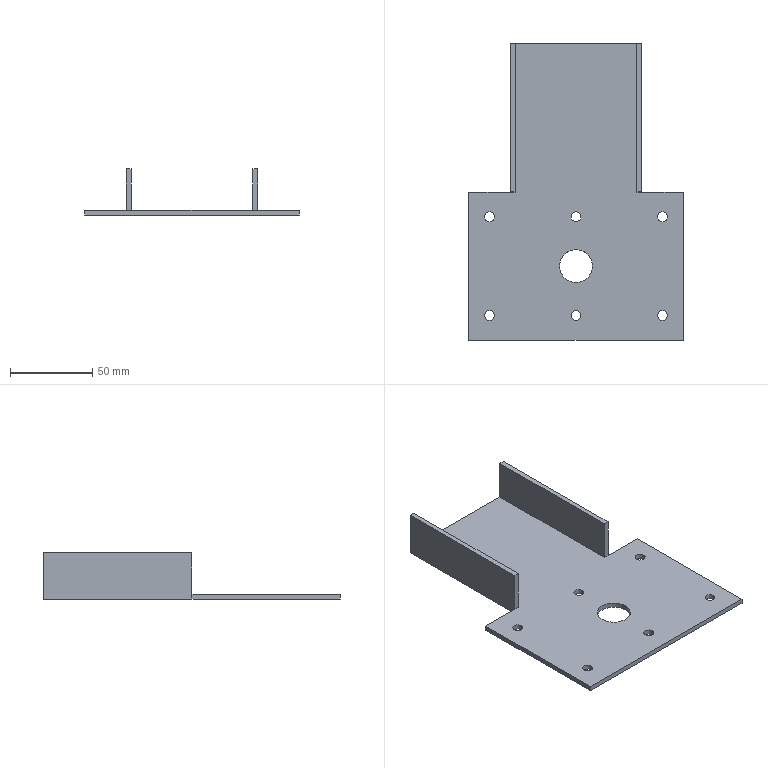Part | SolidWorks | features ICE 2, Extrusion 1 | 1 solid | 30 faces | box 130 x 180 x 28 mm | volume 68749 mm3 | plane 16 | cylinder 14 | commonest cylinder face diameters 6 x12 20 x2
STEP:
#1=CARTESIAN_POINT('',(-15.5,75.,3.));
#2=VERTEX_POINT('',#1);
#3=CARTESIAN_POINT('',(-9.5,75.,3.));
#4=VERTEX_POINT('',#3);
#5=CARTESIAN_POINT('',(-12.5,75.,3.));
#6=DIRECTION('',(0.,0.,1.));
#7=DIRECTION('',(1.,0.,0.));
#8=AXIS2_PLACEMENT_3D('',#5,#6,#7);
#9=CIRCLE('',#8,3.);
#10=EDGE_CURVE('',#2,#4,#9,.T.);
#11=ORIENTED_EDGE('',*,*,#10,.T.);
#12=CARTESIAN_POINT('',(-9.5,75.,0.));
#13=VERTEX_POINT('',#12);
#14=CARTESIAN_POINT('',(-9.5,75.,25.));
#15=DIRECTION('',(0.,0.,-1.));
#16=VECTOR('',#15,1000.);
#17=LINE('',#14,#16);
#18=EDGE_CURVE('',#4,#13,#17,.T.);
#19=ORIENTED_EDGE('',*,*,#18,.T.);
#20=CARTESIAN_POINT('',(-15.5,75.,0.));
#21=VERTEX_POINT('',#20);
#22=CARTESIAN_POINT('',(-12.5,75.,0.));
#23=DIRECTION('',(0.,0.,-1.));
#24=DIRECTION('',(-1.,0.,0.));
#25=AXIS2_PLACEMENT_3D('',#22,#23,#24);
#26=CIRCLE('',#25,3.);
#27=EDGE_CURVE('',#13,#21,#26,.T.);
#28=ORIENTED_EDGE('',*,*,#27,.T.);
#29=CARTESIAN_POINT('',(-15.5,75.,25.));
#30=DIRECTION('',(0.,0.,-1.));
#31=VECTOR('',#30,1000.);
#32=LINE('',#29,#31);
#33=EDGE_CURVE('',#2,#21,#32,.T.);
#34=ORIENTED_EDGE('',*,*,#33,.F.);
#35=EDGE_LOOP('',(#11,#19,#28,#34));
#36=FACE_OUTER_BOUND('',#35,.T.);
#37=CARTESIAN_POINT('',(-12.5,75.,25.));
#38=DIRECTION('',(0.,0.,-1.));
#39=DIRECTION('',(-1.,0.,0.));
#40=AXIS2_PLACEMENT_3D('',#37,#38,#39);
#41=CYLINDRICAL_SURFACE('',#40,3.);
#42=ADVANCED_FACE('',(#36),#41,.F.);
#43=CARTESIAN_POINT('',(-68.,75.,3.));
#44=VERTEX_POINT('',#43);
#45=CARTESIAN_POINT('',(-62.,75.,3.));
#46=VERTEX_POINT('',#45);
#47=CARTESIAN_POINT('',(-65.,75.,3.));
#48=DIRECTION('',(0.,0.,1.));
#49=DIRECTION('',(1.,0.,0.));
#50=AXIS2_PLACEMENT_3D('',#47,#48,#49);
#51=CIRCLE('',#50,3.);
#52=EDGE_CURVE('',#44,#46,#51,.T.);
#53=ORIENTED_EDGE('',*,*,#52,.T.);
#54=CARTESIAN_POINT('',(-62.,75.,0.));
#55=VERTEX_POINT('',#54);
#56=CARTESIAN_POINT('',(-62.,75.,25.));
#57=DIRECTION('',(0.,0.,-1.));
#58=VECTOR('',#57,1000.);
#59=LINE('',#56,#58);
#60=EDGE_CURVE('',#46,#55,#59,.T.);
#61=ORIENTED_EDGE('',*,*,#60,.T.);
#62=CARTESIAN_POINT('',(-68.,75.,0.));
#63=VERTEX_POINT('',#62);
#64=CARTESIAN_POINT('',(-65.,75.,0.));
#65=DIRECTION('',(0.,0.,-1.));
#66=DIRECTION('',(-1.,0.,0.));
#67=AXIS2_PLACEMENT_3D('',#64,#65,#66);
#68=CIRCLE('',#67,3.);
#69=EDGE_CURVE('',#55,#63,#68,.T.);
#70=ORIENTED_EDGE('',*,*,#69,.T.);
#71=CARTESIAN_POINT('',(-68.,75.,25.));
#72=DIRECTION('',(0.,0.,-1.));
#73=VECTOR('',#72,1000.);
#74=LINE('',#71,#73);
#75=EDGE_CURVE('',#44,#63,#74,.T.);
#76=ORIENTED_EDGE('',*,*,#75,.F.);
#77=EDGE_LOOP('',(#53,#61,#70,#76));
#78=FACE_OUTER_BOUND('',#77,.T.);
#79=CARTESIAN_POINT('',(-65.,75.,25.));
#80=DIRECTION('',(0.,0.,-1.));
#81=DIRECTION('',(-1.,0.,0.));
#82=AXIS2_PLACEMENT_3D('',#79,#80,#81);
#83=CYLINDRICAL_SURFACE('',#82,3.);
#84=ADVANCED_FACE('',(#78),#83,.F.);
#85=CARTESIAN_POINT('',(-120.5,75.,3.));
#86=VERTEX_POINT('',#85);
#87=CARTESIAN_POINT('',(-114.5,75.,3.));
#88=VERTEX_POINT('',#87);
#89=CARTESIAN_POINT('',(-117.5,75.,3.));
#90=DIRECTION('',(0.,0.,1.));
#91=DIRECTION('',(1.,0.,0.));
#92=AXIS2_PLACEMENT_3D('',#89,#90,#91);
#93=CIRCLE('',#92,3.);
#94=EDGE_CURVE('',#86,#88,#93,.T.);
#95=ORIENTED_EDGE('',*,*,#94,.T.);
#96=CARTESIAN_POINT('',(-114.5,75.,0.));
#97=VERTEX_POINT('',#96);
#98=CARTESIAN_POINT('',(-114.5,75.,25.));
#99=DIRECTION('',(0.,0.,-1.));
#100=VECTOR('',#99,1000.);
#101=LINE('',#98,#100);
#102=EDGE_CURVE('',#88,#97,#101,.T.);
#103=ORIENTED_EDGE('',*,*,#102,.T.);
#104=CARTESIAN_POINT('',(-120.5,75.,0.));
#105=VERTEX_POINT('',#104);
#106=CARTESIAN_POINT('',(-117.5,75.,0.));
#107=DIRECTION('',(0.,0.,-1.));
#108=DIRECTION('',(-1.,0.,0.));
#109=AXIS2_PLACEMENT_3D('',#106,#107,#108);
#110=CIRCLE('',#109,3.);
#111=EDGE_CURVE('',#97,#105,#110,.T.);
#112=ORIENTED_EDGE('',*,*,#111,.T.);
#113=CARTESIAN_POINT('',(-120.5,75.,25.));
#114=DIRECTION('',(0.,0.,-1.));
#115=VECTOR('',#114,1000.);
#116=LINE('',#113,#115);
#117=EDGE_CURVE('',#86,#105,#116,.T.);
#118=ORIENTED_EDGE('',*,*,#117,.F.);
#119=EDGE_LOOP('',(#95,#103,#112,#118));
#120=FACE_OUTER_BOUND('',#119,.T.);
#121=CARTESIAN_POINT('',(-117.5,75.,25.));
#122=DIRECTION('',(0.,0.,-1.));
#123=DIRECTION('',(-1.,0.,0.));
#124=AXIS2_PLACEMENT_3D('',#121,#122,#123);
#125=CYLINDRICAL_SURFACE('',#124,3.);
#126=ADVANCED_FACE('',(#120),#125,.F.);
#127=CARTESIAN_POINT('',(-120.5,15.,3.));
#128=VERTEX_POINT('',#127);
#129=CARTESIAN_POINT('',(-114.5,15.,3.));
#130=VERTEX_POINT('',#129);
#131=CARTESIAN_POINT('',(-117.5,15.,3.));
#132=DIRECTION('',(0.,0.,1.));
#133=DIRECTION('',(1.,0.,0.));
#134=AXIS2_PLACEMENT_3D('',#131,#132,#133);
#135=CIRCLE('',#134,3.);
#136=EDGE_CURVE('',#128,#130,#135,.T.);
#137=ORIENTED_EDGE('',*,*,#136,.T.);
#138=CARTESIAN_POINT('',(-114.5,15.,0.));
#139=VERTEX_POINT('',#138);
#140=CARTESIAN_POINT('',(-114.5,15.,25.));
#141=DIRECTION('',(0.,0.,-1.));
#142=VECTOR('',#141,1000.);
#143=LINE('',#140,#142);
#144=EDGE_CURVE('',#130,#139,#143,.T.);
#145=ORIENTED_EDGE('',*,*,#144,.T.);
#146=CARTESIAN_POINT('',(-120.5,15.,0.));
#147=VERTEX_POINT('',#146);
#148=CARTESIAN_POINT('',(-117.5,15.,0.));
#149=DIRECTION('',(0.,0.,-1.));
#150=DIRECTION('',(-1.,0.,0.));
#151=AXIS2_PLACEMENT_3D('',#148,#149,#150);
#152=CIRCLE('',#151,3.);
#153=EDGE_CURVE('',#139,#147,#152,.T.);
#154=ORIENTED_EDGE('',*,*,#153,.T.);
#155=CARTESIAN_POINT('',(-120.5,15.,25.));
#156=DIRECTION('',(0.,0.,-1.));
#157=VECTOR('',#156,1000.);
#158=LINE('',#155,#157);
#159=EDGE_CURVE('',#128,#147,#158,.T.);
#160=ORIENTED_EDGE('',*,*,#159,.F.);
#161=EDGE_LOOP('',(#137,#145,#154,#160));
#162=FACE_OUTER_BOUND('',#161,.T.);
#163=CARTESIAN_POINT('',(-117.5,15.,25.));
#164=DIRECTION('',(0.,0.,-1.));
#165=DIRECTION('',(-1.,0.,0.));
#166=AXIS2_PLACEMENT_3D('',#163,#164,#165);
#167=CYLINDRICAL_SURFACE('',#166,3.);
#168=ADVANCED_FACE('',(#162),#167,.F.);
#169=CARTESIAN_POINT('',(-68.,15.,3.));
#170=VERTEX_POINT('',#169);
#171=CARTESIAN_POINT('',(-62.,15.,3.));
#172=VERTEX_POINT('',#171);
#173=CARTESIAN_POINT('',(-65.,15.,3.));
#174=DIRECTION('',(0.,0.,1.));
#175=DIRECTION('',(1.,0.,0.));
#176=AXIS2_PLACEMENT_3D('',#173,#174,#175);
#177=CIRCLE('',#176,3.);
#178=EDGE_CURVE('',#170,#172,#177,.T.);
#179=ORIENTED_EDGE('',*,*,#178,.T.);
#180=CARTESIAN_POINT('',(-62.,15.,0.));
#181=VERTEX_POINT('',#180);
#182=CARTESIAN_POINT('',(-62.,15.,25.));
#183=DIRECTION('',(0.,0.,-1.));
#184=VECTOR('',#183,1000.);
#185=LINE('',#182,#184);
#186=EDGE_CURVE('',#172,#181,#185,.T.);
#187=ORIENTED_EDGE('',*,*,#186,.T.);
#188=CARTESIAN_POINT('',(-68.,15.,0.));
#189=VERTEX_POINT('',#188);
#190=CARTESIAN_POINT('',(-65.,15.,0.));
#191=DIRECTION('',(0.,0.,-1.));
#192=DIRECTION('',(-1.,0.,0.));
#193=AXIS2_PLACEMENT_3D('',#190,#191,#192);
#194=CIRCLE('',#193,3.);
#195=EDGE_CURVE('',#181,#189,#194,.T.);
#196=ORIENTED_EDGE('',*,*,#195,.T.);
#197=CARTESIAN_POINT('',(-68.,15.,25.));
#198=DIRECTION('',(0.,0.,-1.));
#199=VECTOR('',#198,1000.);
#200=LINE('',#197,#199);
#201=EDGE_CURVE('',#170,#189,#200,.T.);
#202=ORIENTED_EDGE('',*,*,#201,.F.);
#203=EDGE_LOOP('',(#179,#187,#196,#202));
#204=FACE_OUTER_BOUND('',#203,.T.);
#205=CARTESIAN_POINT('',(-65.,15.,25.));
#206=DIRECTION('',(0.,0.,-1.));
#207=DIRECTION('',(-1.,0.,0.));
#208=AXIS2_PLACEMENT_3D('',#205,#206,#207);
#209=CYLINDRICAL_SURFACE('',#208,3.);
#210=ADVANCED_FACE('',(#204),#209,.F.);
#211=CARTESIAN_POINT('',(-15.5,15.,3.));
#212=VERTEX_POINT('',#211);
#213=CARTESIAN_POINT('',(-9.5,15.,3.));
#214=VERTEX_POINT('',#213);
#215=CARTESIAN_POINT('',(-12.5,15.,3.));
#216=DIRECTION('',(0.,0.,1.));
#217=DIRECTION('',(1.,0.,0.));
#218=AXIS2_PLACEMENT_3D('',#215,#216,#217);
#219=CIRCLE('',#218,3.);
#220=EDGE_CURVE('',#212,#214,#219,.T.);
#221=ORIENTED_EDGE('',*,*,#220,.T.);
#222=CARTESIAN_POINT('',(-9.5,15.,0.));
#223=VERTEX_POINT('',#222);
#224=CARTESIAN_POINT('',(-9.5,15.,25.));
#225=DIRECTION('',(0.,0.,-1.));
#226=VECTOR('',#225,1000.);
#227=LINE('',#224,#226);
#228=EDGE_CURVE('',#214,#223,#227,.T.);
#229=ORIENTED_EDGE('',*,*,#228,.T.);
#230=CARTESIAN_POINT('',(-15.5,15.,0.));
#231=VERTEX_POINT('',#230);
#232=CARTESIAN_POINT('',(-12.5,15.,0.));
#233=DIRECTION('',(0.,0.,-1.));
#234=DIRECTION('',(-1.,0.,0.));
#235=AXIS2_PLACEMENT_3D('',#232,#233,#234);
#236=CIRCLE('',#235,3.);
#237=EDGE_CURVE('',#223,#231,#236,.T.);
#238=ORIENTED_EDGE('',*,*,#237,.T.);
#239=CARTESIAN_POINT('',(-15.5,15.,25.));
#240=DIRECTION('',(0.,0.,-1.));
#241=VECTOR('',#240,1000.);
#242=LINE('',#239,#241);
#243=EDGE_CURVE('',#212,#231,#242,.T.);
#244=ORIENTED_EDGE('',*,*,#243,.F.);
#245=EDGE_LOOP('',(#221,#229,#238,#244));
#246=FACE_OUTER_BOUND('',#245,.T.);
#247=CARTESIAN_POINT('',(-12.5,15.,25.));
#248=DIRECTION('',(0.,0.,-1.));
#249=DIRECTION('',(-1.,0.,0.));
#250=AXIS2_PLACEMENT_3D('',#247,#248,#249);
#251=CYLINDRICAL_SURFACE('',#250,3.);
#252=ADVANCED_FACE('',(#246),#251,.F.);
#253=CARTESIAN_POINT('',(-75.,45.,3.));
#254=VERTEX_POINT('',#253);
#255=CARTESIAN_POINT('',(-55.,45.,3.));
#256=VERTEX_POINT('',#255);
#257=CARTESIAN_POINT('',(-65.,45.,3.));
#258=DIRECTION('',(0.,0.,1.));
#259=DIRECTION('',(1.,0.,0.));
#260=AXIS2_PLACEMENT_3D('',#257,#258,#259);
#261=CIRCLE('',#260,10.);
#262=EDGE_CURVE('',#254,#256,#261,.T.);
#263=ORIENTED_EDGE('',*,*,#262,.T.);
#264=CARTESIAN_POINT('',(-55.,45.,0.));
#265=VERTEX_POINT('',#264);
#266=CARTESIAN_POINT('',(-55.,45.,25.));
#267=DIRECTION('',(0.,0.,-1.));
#268=VECTOR('',#267,1000.);
#269=LINE('',#266,#268);
#270=EDGE_CURVE('',#256,#265,#269,.T.);
#271=ORIENTED_EDGE('',*,*,#270,.T.);
#272=CARTESIAN_POINT('',(-75.,45.,0.));
#273=VERTEX_POINT('',#272);
#274=CARTESIAN_POINT('',(-65.,45.,0.));
#275=DIRECTION('',(0.,0.,-1.));
#276=DIRECTION('',(-1.,0.,0.));
#277=AXIS2_PLACEMENT_3D('',#274,#275,#276);
#278=CIRCLE('',#277,10.);
#279=EDGE_CURVE('',#265,#273,#278,.T.);
#280=ORIENTED_EDGE('',*,*,#279,.T.);
#281=CARTESIAN_POINT('',(-75.,45.,25.));
#282=DIRECTION('',(0.,0.,-1.));
#283=VECTOR('',#282,1000.);
#284=LINE('',#281,#283);
#285=EDGE_CURVE('',#254,#273,#284,.T.);
#286=ORIENTED_EDGE('',*,*,#285,.F.);
#287=EDGE_LOOP('',(#263,#271,#280,#286));
#288=FACE_OUTER_BOUND('',#287,.T.);
#289=CARTESIAN_POINT('',(-65.,45.,25.));
#290=DIRECTION('',(0.,0.,-1.));
#291=DIRECTION('',(-1.,0.,0.));
#292=AXIS2_PLACEMENT_3D('',#289,#290,#291);
#293=CYLINDRICAL_SURFACE('',#292,10.);
#294=ADVANCED_FACE('',(#288),#293,.F.);
#295=ORIENTED_EDGE('',*,*,#10,.F.);
#296=CARTESIAN_POINT('',(-12.5,75.,3.));
#297=DIRECTION('',(0.,0.,1.));
#298=DIRECTION('',(1.,0.,0.));
#299=AXIS2_PLACEMENT_3D('',#296,#297,#298);
#300=CIRCLE('',#299,3.);
#301=EDGE_CURVE('',#4,#2,#300,.T.);
#302=ORIENTED_EDGE('',*,*,#301,.F.);
#303=EDGE_LOOP('',(#295,#302));
#304=FACE_BOUND('',#303,.T.);
#305=ORIENTED_EDGE('',*,*,#52,.F.);
#306=CARTESIAN_POINT('',(-65.,75.,3.));
#307=DIRECTION('',(0.,0.,1.));
#308=DIRECTION('',(1.,0.,0.));
#309=AXIS2_PLACEMENT_3D('',#306,#307,#308);
#310=CIRCLE('',#309,3.);
#311=EDGE_CURVE('',#46,#44,#310,.T.);
#312=ORIENTED_EDGE('',*,*,#311,.F.);
#313=EDGE_LOOP('',(#305,#312));
#314=FACE_BOUND('',#313,.T.);
#315=ORIENTED_EDGE('',*,*,#94,.F.);
#316=CARTESIAN_POINT('',(-117.5,75.,3.));
#317=DIRECTION('',(0.,0.,1.));
#318=DIRECTION('',(1.,0.,0.));
#319=AXIS2_PLACEMENT_3D('',#316,#317,#318);
#320=CIRCLE('',#319,3.);
#321=EDGE_CURVE('',#88,#86,#320,.T.);
#322=ORIENTED_EDGE('',*,*,#321,.F.);
#323=EDGE_LOOP('',(#315,#322));
#324=FACE_BOUND('',#323,.T.);
#325=ORIENTED_EDGE('',*,*,#136,.F.);
#326=CARTESIAN_POINT('',(-117.5,15.,3.));
#327=DIRECTION('',(0.,0.,1.));
#328=DIRECTION('',(1.,0.,0.));
#329=AXIS2_PLACEMENT_3D('',#326,#327,#328);
#330=CIRCLE('',#329,3.);
#331=EDGE_CURVE('',#130,#128,#330,.T.);
#332=ORIENTED_EDGE('',*,*,#331,.F.);
#333=EDGE_LOOP('',(#325,#332));
#334=FACE_BOUND('',#333,.T.);
#335=ORIENTED_EDGE('',*,*,#178,.F.);
#336=CARTESIAN_POINT('',(-65.,15.,3.));
#337=DIRECTION('',(0.,0.,1.));
#338=DIRECTION('',(1.,0.,0.));
#339=AXIS2_PLACEMENT_3D('',#336,#337,#338);
#340=CIRCLE('',#339,3.);
#341=EDGE_CURVE('',#172,#170,#340,.T.);
#342=ORIENTED_EDGE('',*,*,#341,.F.);
#343=EDGE_LOOP('',(#335,#342));
#344=FACE_BOUND('',#343,.T.);
#345=ORIENTED_EDGE('',*,*,#220,.F.);
#346=CARTESIAN_POINT('',(-12.5,15.,3.));
#347=DIRECTION('',(0.,0.,1.));
#348=DIRECTION('',(1.,0.,0.));
#349=AXIS2_PLACEMENT_3D('',#346,#347,#348);
#350=CIRCLE('',#349,3.);
#351=EDGE_CURVE('',#214,#212,#350,.T.);
#352=ORIENTED_EDGE('',*,*,#351,.F.);
#353=EDGE_LOOP('',(#345,#352));
#354=FACE_BOUND('',#353,.T.);
#355=ORIENTED_EDGE('',*,*,#262,.F.);
#356=CARTESIAN_POINT('',(-65.,45.,3.));
#357=DIRECTION('',(0.,0.,1.));
#358=DIRECTION('',(1.,0.,0.));
#359=AXIS2_PLACEMENT_3D('',#356,#357,#358);
#360=CIRCLE('',#359,10.);
#361=EDGE_CURVE('',#256,#254,#360,.T.);
#362=ORIENTED_EDGE('',*,*,#361,.F.);
#363=EDGE_LOOP('',(#355,#362));
#364=FACE_BOUND('',#363,.T.);
#365=CARTESIAN_POINT('',(-28.,90.,3.));
#366=VERTEX_POINT('',#365);
#367=CARTESIAN_POINT('',(-25.,90.,3.));
#368=VERTEX_POINT('',#367);
#369=CARTESIAN_POINT('',(-28.,90.,3.));
#370=DIRECTION('',(1.,0.,0.));
#371=VECTOR('',#370,1000.);
#372=LINE('',#369,#371);
#373=EDGE_CURVE('',#366,#368,#372,.T.);
#374=ORIENTED_EDGE('',*,*,#373,.F.);
#375=CARTESIAN_POINT('',(-28.,180.,3.));
#376=VERTEX_POINT('',#375);
#377=CARTESIAN_POINT('',(-28.,180.,3.));
#378=DIRECTION('',(0.,-1.,0.));
#379=VECTOR('',#378,1000.);
#380=LINE('',#377,#379);
#381=EDGE_CURVE('',#376,#366,#380,.T.);
#382=ORIENTED_EDGE('',*,*,#381,.F.);
#383=CARTESIAN_POINT('',(-102.,180.,3.));
#384=VERTEX_POINT('',#383);
#385=CARTESIAN_POINT('',(0.,180.,3.));
#386=DIRECTION('',(1.,0.,0.));
#387=VECTOR('',#386,1000.);
#388=LINE('',#385,#387);
#389=EDGE_CURVE('',#384,#376,#388,.T.);
#390=ORIENTED_EDGE('',*,*,#389,.F.);
#391=CARTESIAN_POINT('',(-102.,90.,3.));
#392=VERTEX_POINT('',#391);
#393=CARTESIAN_POINT('',(-102.,180.,3.));
#394=DIRECTION('',(0.,1.,0.));
#395=VECTOR('',#394,1000.);
#396=LINE('',#393,#395);
#397=EDGE_CURVE('',#392,#384,#396,.T.);
#398=ORIENTED_EDGE('',*,*,#397,.F.);
#399=CARTESIAN_POINT('',(-105.,90.,3.));
#400=VERTEX_POINT('',#399);
#401=CARTESIAN_POINT('',(-105.,90.,3.));
#402=DIRECTION('',(1.,0.,0.));
#403=VECTOR('',#402,1000.);
#404=LINE('',#401,#403);
#405=EDGE_CURVE('',#400,#392,#404,.T.);
#406=ORIENTED_EDGE('',*,*,#405,.F.);
#407=CARTESIAN_POINT('',(-130.,90.,3.));
#408=VERTEX_POINT('',#407);
#409=CARTESIAN_POINT('',(0.,90.,3.));
#410=DIRECTION('',(-1.,0.,0.));
#411=VECTOR('',#410,1000.);
#412=LINE('',#409,#411);
#413=EDGE_CURVE('',#400,#408,#412,.T.);
#414=ORIENTED_EDGE('',*,*,#413,.T.);
#415=CARTESIAN_POINT('',(-130.,0.,3.));
#416=VERTEX_POINT('',#415);
#417=CARTESIAN_POINT('',(-130.,0.,3.));
#418=DIRECTION('',(0.,1.,0.));
#419=VECTOR('',#418,1000.);
#420=LINE('',#417,#419);
#421=EDGE_CURVE('',#416,#408,#420,.T.);
#422=ORIENTED_EDGE('',*,*,#421,.F.);
#423=CARTESIAN_POINT('',(0.,0.,3.));
#424=VERTEX_POINT('',#423);
#425=CARTESIAN_POINT('',(0.,0.,3.));
#426=DIRECTION('',(-1.,0.,0.));
#427=VECTOR('',#426,1000.);
#428=LINE('',#425,#427);
#429=EDGE_CURVE('',#424,#416,#428,.T.);
#430=ORIENTED_EDGE('',*,*,#429,.F.);
#431=CARTESIAN_POINT('',(0.,90.,3.));
#432=VERTEX_POINT('',#431);
#433=CARTESIAN_POINT('',(0.,0.,3.));
#434=DIRECTION('',(0.,-1.,0.));
#435=VECTOR('',#434,1000.);
#436=LINE('',#433,#435);
#437=EDGE_CURVE('',#432,#424,#436,.T.);
#438=ORIENTED_EDGE('',*,*,#437,.F.);
#439=CARTESIAN_POINT('',(0.,90.,3.));
#440=DIRECTION('',(-1.,0.,0.));
#441=VECTOR('',#440,1000.);
#442=LINE('',#439,#441);
#443=EDGE_CURVE('',#432,#368,#442,.T.);
#444=ORIENTED_EDGE('',*,*,#443,.T.);
#445=EDGE_LOOP('',(#374,#382,#390,#398,#406,#414,#422,#430,#438,#444));
#446=FACE_OUTER_BOUND('',#445,.T.);
#447=CARTESIAN_POINT('',(0.,0.,3.));
#448=DIRECTION('',(0.,0.,1.));
#449=DIRECTION('',(1.,0.,0.));
#450=AXIS2_PLACEMENT_3D('',#447,#448,#449);
#451=PLANE('',#450);
#452=ADVANCED_FACE('',(#304,#314,#324,#334,#344,#354,#364,#446),#451,.T.);
#453=CARTESIAN_POINT('',(-105.,180.,0.));
#454=VERTEX_POINT('',#453);
#455=CARTESIAN_POINT('',(-25.,180.,0.));
#456=VERTEX_POINT('',#455);
#457=CARTESIAN_POINT('',(0.,180.,0.));
#458=DIRECTION('',(1.,0.,0.));
#459=VECTOR('',#458,1000.);
#460=LINE('',#457,#459);
#461=EDGE_CURVE('',#454,#456,#460,.T.);
#462=ORIENTED_EDGE('',*,*,#461,.F.);
#463=CARTESIAN_POINT('',(-105.,180.,28.));
#464=VERTEX_POINT('',#463);
#465=CARTESIAN_POINT('',(-105.,180.,3.));
#466=DIRECTION('',(0.,0.,-1.));
#467=VECTOR('',#466,1000.);
#468=LINE('',#465,#467);
#469=EDGE_CURVE('',#464,#454,#468,.T.);
#470=ORIENTED_EDGE('',*,*,#469,.F.);
#471=CARTESIAN_POINT('',(-102.,180.,28.));
#472=VERTEX_POINT('',#471);
#473=CARTESIAN_POINT('',(-105.,180.,28.));
#474=DIRECTION('',(-1.,0.,0.));
#475=VECTOR('',#474,1000.);
#476=LINE('',#473,#475);
#477=EDGE_CURVE('',#472,#464,#476,.T.);
#478=ORIENTED_EDGE('',*,*,#477,.F.);
#479=CARTESIAN_POINT('',(-102.,180.,28.));
#480=DIRECTION('',(0.,0.,-1.));
#481=VECTOR('',#480,1000.);
#482=LINE('',#479,#481);
#483=EDGE_CURVE('',#472,#384,#482,.T.);
#484=ORIENTED_EDGE('',*,*,#483,.T.);
#485=ORIENTED_EDGE('',*,*,#389,.T.);
#486=CARTESIAN_POINT('',(-28.,180.,28.));
#487=VERTEX_POINT('',#486);
#488=CARTESIAN_POINT('',(-28.,180.,28.));
#489=DIRECTION('',(0.,0.,-1.));
#490=VECTOR('',#489,1000.);
#491=LINE('',#488,#490);
#492=EDGE_CURVE('',#487,#376,#491,.T.);
#493=ORIENTED_EDGE('',*,*,#492,.F.);
#494=CARTESIAN_POINT('',(-25.,180.,28.));
#495=VERTEX_POINT('',#494);
#496=CARTESIAN_POINT('',(-28.,180.,28.));
#497=DIRECTION('',(-1.,0.,0.));
#498=VECTOR('',#497,1000.);
#499=LINE('',#496,#498);
#500=EDGE_CURVE('',#495,#487,#499,.T.);
#501=ORIENTED_EDGE('',*,*,#500,.F.);
#502=CARTESIAN_POINT('',(-25.,180.,3.));
#503=DIRECTION('',(0.,0.,-1.));
#504=VECTOR('',#503,1000.);
#505=LINE('',#502,#504);
#506=EDGE_CURVE('',#495,#456,#505,.T.);
#507=ORIENTED_EDGE('',*,*,#506,.T.);
#508=EDGE_LOOP('',(#462,#470,#478,#484,#485,#493,#501,#507));
#509=FACE_OUTER_BOUND('',#508,.T.);
#510=CARTESIAN_POINT('',(0.,180.,3.));
#511=DIRECTION('',(0.,1.,0.));
#512=DIRECTION('',(0.,0.,1.));
#513=AXIS2_PLACEMENT_3D('',#510,#511,#512);
#514=PLANE('',#513);
#515=ADVANCED_FACE('',(#509),#514,.T.);
#516=CARTESIAN_POINT('',(-105.,90.,0.));
#517=VERTEX_POINT('',#516);
#518=CARTESIAN_POINT('',(-105.,0.,0.));
#519=DIRECTION('',(0.,-1.,0.));
#520=VECTOR('',#519,1000.);
#521=LINE('',#518,#520);
#522=EDGE_CURVE('',#454,#517,#521,.T.);
#523=ORIENTED_EDGE('',*,*,#522,.T.);
#524=CARTESIAN_POINT('',(-105.,90.,3.));
#525=DIRECTION('',(0.,0.,-1.));
#526=VECTOR('',#525,1000.);
#527=LINE('',#524,#526);
#528=EDGE_CURVE('',#400,#517,#527,.T.);
#529=ORIENTED_EDGE('',*,*,#528,.F.);
#530=CARTESIAN_POINT('',(-105.,90.,28.));
#531=VERTEX_POINT('',#530);
#532=CARTESIAN_POINT('',(-105.,90.,28.));
#533=DIRECTION('',(0.,0.,-1.));
#534=VECTOR('',#533,1000.);
#535=LINE('',#532,#534);
#536=EDGE_CURVE('',#531,#400,#535,.T.);
#537=ORIENTED_EDGE('',*,*,#536,.F.);
#538=CARTESIAN_POINT('',(-105.,180.,28.));
#539=DIRECTION('',(0.,-1.,0.));
#540=VECTOR('',#539,1000.);
#541=LINE('',#538,#540);
#542=EDGE_CURVE('',#464,#531,#541,.T.);
#543=ORIENTED_EDGE('',*,*,#542,.F.);
#544=ORIENTED_EDGE('',*,*,#469,.T.);
#545=EDGE_LOOP('',(#523,#529,#537,#543,#544));
#546=FACE_OUTER_BOUND('',#545,.T.);
#547=CARTESIAN_POINT('',(-105.,0.,3.));
#548=DIRECTION('',(1.,0.,0.));
#549=DIRECTION('',(0.,0.,-1.));
#550=AXIS2_PLACEMENT_3D('',#547,#548,#549);
#551=PLANE('',#550);
#552=ADVANCED_FACE('',(#546),#551,.F.);
#553=CARTESIAN_POINT('',(-130.,90.,0.));
#554=VERTEX_POINT('',#553);
#555=CARTESIAN_POINT('',(0.,90.,0.));
#556=DIRECTION('',(-1.,0.,0.));
#557=VECTOR('',#556,1000.);
#558=LINE('',#555,#557);
#559=EDGE_CURVE('',#517,#554,#558,.T.);
#560=ORIENTED_EDGE('',*,*,#559,.T.);
#561=CARTESIAN_POINT('',(-130.,90.,3.));
#562=DIRECTION('',(0.,0.,-1.));
#563=VECTOR('',#562,1000.);
#564=LINE('',#561,#563);
#565=EDGE_CURVE('',#408,#554,#564,.T.);
#566=ORIENTED_EDGE('',*,*,#565,.F.);
#567=ORIENTED_EDGE('',*,*,#413,.F.);
#568=ORIENTED_EDGE('',*,*,#528,.T.);
#569=EDGE_LOOP('',(#560,#566,#567,#568));
#570=FACE_OUTER_BOUND('',#569,.T.);
#571=CARTESIAN_POINT('',(0.,90.,3.));
#572=DIRECTION('',(0.,-1.,0.));
#573=DIRECTION('',(1.,0.,0.));
#574=AXIS2_PLACEMENT_3D('',#571,#572,#573);
#575=PLANE('',#574);
#576=ADVANCED_FACE('',(#570),#575,.F.);
#577=CARTESIAN_POINT('',(-130.,0.,0.));
#578=VERTEX_POINT('',#577);
#579=CARTESIAN_POINT('',(-130.,0.,0.));
#580=DIRECTION('',(0.,1.,0.));
#581=VECTOR('',#580,1000.);
#582=LINE('',#579,#581);
#583=EDGE_CURVE('',#578,#554,#582,.T.);
#584=ORIENTED_EDGE('',*,*,#583,.F.);
#585=CARTESIAN_POINT('',(-130.,0.,3.));
#586=DIRECTION('',(0.,0.,-1.));
#587=VECTOR('',#586,1000.);
#588=LINE('',#585,#587);
#589=EDGE_CURVE('',#416,#578,#588,.T.);
#590=ORIENTED_EDGE('',*,*,#589,.F.);
#591=ORIENTED_EDGE('',*,*,#421,.T.);
#592=ORIENTED_EDGE('',*,*,#565,.T.);
#593=EDGE_LOOP('',(#584,#590,#591,#592));
#594=FACE_OUTER_BOUND('',#593,.T.);
#595=CARTESIAN_POINT('',(-130.,0.,3.));
#596=DIRECTION('',(-1.,0.,0.));
#597=DIRECTION('',(0.,0.,1.));
#598=AXIS2_PLACEMENT_3D('',#595,#596,#597);
#599=PLANE('',#598);
#600=ADVANCED_FACE('',(#594),#599,.T.);
#601=CARTESIAN_POINT('',(0.,0.,0.));
#602=VERTEX_POINT('',#601);
#603=CARTESIAN_POINT('',(0.,0.,0.));
#604=DIRECTION('',(-1.,0.,0.));
#605=VECTOR('',#604,1000.);
#606=LINE('',#603,#605);
#607=EDGE_CURVE('',#602,#578,#606,.T.);
#608=ORIENTED_EDGE('',*,*,#607,.F.);
#609=CARTESIAN_POINT('',(0.,0.,3.));
#610=DIRECTION('',(0.,0.,-1.));
#611=VECTOR('',#610,1000.);
#612=LINE('',#609,#611);
#613=EDGE_CURVE('',#424,#602,#612,.T.);
#614=ORIENTED_EDGE('',*,*,#613,.F.);
#615=ORIENTED_EDGE('',*,*,#429,.T.);
#616=ORIENTED_EDGE('',*,*,#589,.T.);
#617=EDGE_LOOP('',(#608,#614,#615,#616));
#618=FACE_OUTER_BOUND('',#617,.T.);
#619=CARTESIAN_POINT('',(0.,0.,3.));
#620=DIRECTION('',(0.,-1.,0.));
#621=DIRECTION('',(1.,0.,0.));
#622=AXIS2_PLACEMENT_3D('',#619,#620,#621);
#623=PLANE('',#622);
#624=ADVANCED_FACE('',(#618),#623,.T.);
#625=CARTESIAN_POINT('',(0.,90.,0.));
#626=VERTEX_POINT('',#625);
#627=CARTESIAN_POINT('',(0.,0.,0.));
#628=DIRECTION('',(0.,-1.,0.));
#629=VECTOR('',#628,1000.);
#630=LINE('',#627,#629);
#631=EDGE_CURVE('',#626,#602,#630,.T.);
#632=ORIENTED_EDGE('',*,*,#631,.F.);
#633=CARTESIAN_POINT('',(0.,90.,3.));
#634=DIRECTION('',(0.,0.,-1.));
#635=VECTOR('',#634,1000.);
#636=LINE('',#633,#635);
#637=EDGE_CURVE('',#432,#626,#636,.T.);
#638=ORIENTED_EDGE('',*,*,#637,.F.);
#639=ORIENTED_EDGE('',*,*,#437,.T.);
#640=ORIENTED_EDGE('',*,*,#613,.T.);
#641=EDGE_LOOP('',(#632,#638,#639,#640));
#642=FACE_OUTER_BOUND('',#641,.T.);
#643=CARTESIAN_POINT('',(0.,0.,3.));
#644=DIRECTION('',(1.,0.,0.));
#645=DIRECTION('',(0.,0.,-1.));
#646=AXIS2_PLACEMENT_3D('',#643,#644,#645);
#647=PLANE('',#646);
#648=ADVANCED_FACE('',(#642),#647,.T.);
#649=CARTESIAN_POINT('',(-25.,90.,0.));
#650=VERTEX_POINT('',#649);
#651=CARTESIAN_POINT('',(0.,90.,0.));
#652=DIRECTION('',(-1.,0.,0.));
#653=VECTOR('',#652,1000.);
#654=LINE('',#651,#653);
#655=EDGE_CURVE('',#626,#650,#654,.T.);
#656=ORIENTED_EDGE('',*,*,#655,.T.);
#657=CARTESIAN_POINT('',(-25.,90.,3.));
#658=DIRECTION('',(0.,0.,-1.));
#659=VECTOR('',#658,1000.);
#660=LINE('',#657,#659);
#661=EDGE_CURVE('',#368,#650,#660,.T.);
#662=ORIENTED_EDGE('',*,*,#661,.F.);
#663=ORIENTED_EDGE('',*,*,#443,.F.);
#664=ORIENTED_EDGE('',*,*,#637,.T.);
#665=EDGE_LOOP('',(#656,#662,#663,#664));
#666=FACE_OUTER_BOUND('',#665,.T.);
#667=CARTESIAN_POINT('',(0.,90.,3.));
#668=DIRECTION('',(0.,-1.,0.));
#669=DIRECTION('',(1.,0.,0.));
#670=AXIS2_PLACEMENT_3D('',#667,#668,#669);
#671=PLANE('',#670);
#672=ADVANCED_FACE('',(#666),#671,.F.);
#673=CARTESIAN_POINT('',(-25.,0.,0.));
#674=DIRECTION('',(0.,-1.,0.));
#675=VECTOR('',#674,1000.);
#676=LINE('',#673,#675);
#677=EDGE_CURVE('',#456,#650,#676,.T.);
#678=ORIENTED_EDGE('',*,*,#677,.F.);
#679=ORIENTED_EDGE('',*,*,#506,.F.);
#680=CARTESIAN_POINT('',(-25.,90.,28.));
#681=VERTEX_POINT('',#680);
#682=CARTESIAN_POINT('',(-25.,180.,28.));
#683=DIRECTION('',(0.,1.,0.));
#684=VECTOR('',#683,1000.);
#685=LINE('',#682,#684);
#686=EDGE_CURVE('',#681,#495,#685,.T.);
#687=ORIENTED_EDGE('',*,*,#686,.F.);
#688=CARTESIAN_POINT('',(-25.,90.,28.));
#689=DIRECTION('',(0.,0.,-1.));
#690=VECTOR('',#689,1000.);
#691=LINE('',#688,#690);
#692=EDGE_CURVE('',#681,#368,#691,.T.);
#693=ORIENTED_EDGE('',*,*,#692,.T.);
#694=ORIENTED_EDGE('',*,*,#661,.T.);
#695=EDGE_LOOP('',(#678,#679,#687,#693,#694));
#696=FACE_OUTER_BOUND('',#695,.T.);
#697=CARTESIAN_POINT('',(-25.,0.,3.));
#698=DIRECTION('',(1.,0.,0.));
#699=DIRECTION('',(0.,0.,-1.));
#700=AXIS2_PLACEMENT_3D('',#697,#698,#699);
#701=PLANE('',#700);
#702=ADVANCED_FACE('',(#696),#701,.T.);
#703=CARTESIAN_POINT('',(-12.5,75.,0.));
#704=DIRECTION('',(0.,0.,-1.));
#705=DIRECTION('',(-1.,0.,0.));
#706=AXIS2_PLACEMENT_3D('',#703,#704,#705);
#707=CIRCLE('',#706,3.);
#708=EDGE_CURVE('',#21,#13,#707,.T.);
#709=ORIENTED_EDGE('',*,*,#708,.F.);
#710=ORIENTED_EDGE('',*,*,#27,.F.);
#711=EDGE_LOOP('',(#709,#710));
#712=FACE_BOUND('',#711,.T.);
#713=CARTESIAN_POINT('',(-65.,75.,0.));
#714=DIRECTION('',(0.,0.,-1.));
#715=DIRECTION('',(-1.,0.,0.));
#716=AXIS2_PLACEMENT_3D('',#713,#714,#715);
#717=CIRCLE('',#716,3.);
#718=EDGE_CURVE('',#63,#55,#717,.T.);
#719=ORIENTED_EDGE('',*,*,#718,.F.);
#720=ORIENTED_EDGE('',*,*,#69,.F.);
#721=EDGE_LOOP('',(#719,#720));
#722=FACE_BOUND('',#721,.T.);
#723=CARTESIAN_POINT('',(-117.5,75.,0.));
#724=DIRECTION('',(0.,0.,-1.));
#725=DIRECTION('',(-1.,0.,0.));
#726=AXIS2_PLACEMENT_3D('',#723,#724,#725);
#727=CIRCLE('',#726,3.);
#728=EDGE_CURVE('',#105,#97,#727,.T.);
#729=ORIENTED_EDGE('',*,*,#728,.F.);
#730=ORIENTED_EDGE('',*,*,#111,.F.);
#731=EDGE_LOOP('',(#729,#730));
#732=FACE_BOUND('',#731,.T.);
#733=CARTESIAN_POINT('',(-117.5,15.,0.));
#734=DIRECTION('',(0.,0.,-1.));
#735=DIRECTION('',(-1.,0.,0.));
#736=AXIS2_PLACEMENT_3D('',#733,#734,#735);
#737=CIRCLE('',#736,3.);
#738=EDGE_CURVE('',#147,#139,#737,.T.);
#739=ORIENTED_EDGE('',*,*,#738,.F.);
#740=ORIENTED_EDGE('',*,*,#153,.F.);
#741=EDGE_LOOP('',(#739,#740));
#742=FACE_BOUND('',#741,.T.);
#743=CARTESIAN_POINT('',(-65.,15.,0.));
#744=DIRECTION('',(0.,0.,-1.));
#745=DIRECTION('',(-1.,0.,0.));
#746=AXIS2_PLACEMENT_3D('',#743,#744,#745);
#747=CIRCLE('',#746,3.);
#748=EDGE_CURVE('',#189,#181,#747,.T.);
#749=ORIENTED_EDGE('',*,*,#748,.F.);
#750=ORIENTED_EDGE('',*,*,#195,.F.);
#751=EDGE_LOOP('',(#749,#750));
#752=FACE_BOUND('',#751,.T.);
#753=CARTESIAN_POINT('',(-12.5,15.,0.));
#754=DIRECTION('',(0.,0.,-1.));
#755=DIRECTION('',(-1.,0.,0.));
#756=AXIS2_PLACEMENT_3D('',#753,#754,#755);
#757=CIRCLE('',#756,3.);
#758=EDGE_CURVE('',#231,#223,#757,.T.);
#759=ORIENTED_EDGE('',*,*,#758,.F.);
#760=ORIENTED_EDGE('',*,*,#237,.F.);
#761=EDGE_LOOP('',(#759,#760));
#762=FACE_BOUND('',#761,.T.);
#763=CARTESIAN_POINT('',(-65.,45.,0.));
#764=DIRECTION('',(0.,0.,-1.));
#765=DIRECTION('',(-1.,0.,0.));
#766=AXIS2_PLACEMENT_3D('',#763,#764,#765);
#767=CIRCLE('',#766,10.);
#768=EDGE_CURVE('',#273,#265,#767,.T.);
#769=ORIENTED_EDGE('',*,*,#768,.F.);
#770=ORIENTED_EDGE('',*,*,#279,.F.);
#771=EDGE_LOOP('',(#769,#770));
#772=FACE_BOUND('',#771,.T.);
#773=ORIENTED_EDGE('',*,*,#461,.T.);
#774=ORIENTED_EDGE('',*,*,#677,.T.);
#775=ORIENTED_EDGE('',*,*,#655,.F.);
#776=ORIENTED_EDGE('',*,*,#631,.T.);
#777=ORIENTED_EDGE('',*,*,#607,.T.);
#778=ORIENTED_EDGE('',*,*,#583,.T.);
#779=ORIENTED_EDGE('',*,*,#559,.F.);
#780=ORIENTED_EDGE('',*,*,#522,.F.);
#781=EDGE_LOOP('',(#773,#774,#775,#776,#777,#778,#779,#780));
#782=FACE_OUTER_BOUND('',#781,.T.);
#783=CARTESIAN_POINT('',(0.,0.,0.));
#784=DIRECTION('',(0.,0.,1.));
#785=DIRECTION('',(1.,0.,0.));
#786=AXIS2_PLACEMENT_3D('',#783,#784,#785);
#787=PLANE('',#786);
#788=ADVANCED_FACE('',(#712,#722,#732,#742,#752,#762,#772,#782),#787,.F.);
#789=ORIENTED_EDGE('',*,*,#405,.T.);
#790=CARTESIAN_POINT('',(-102.,90.,28.));
#791=VERTEX_POINT('',#790);
#792=CARTESIAN_POINT('',(-102.,90.,28.));
#793=DIRECTION('',(0.,0.,-1.));
#794=VECTOR('',#793,1000.);
#795=LINE('',#792,#794);
#796=EDGE_CURVE('',#791,#392,#795,.T.);
#797=ORIENTED_EDGE('',*,*,#796,.F.);
#798=CARTESIAN_POINT('',(-105.,90.,28.));
#799=DIRECTION('',(1.,0.,0.));
#800=VECTOR('',#799,1000.);
#801=LINE('',#798,#800);
#802=EDGE_CURVE('',#531,#791,#801,.T.);
#803=ORIENTED_EDGE('',*,*,#802,.F.);
#804=ORIENTED_EDGE('',*,*,#536,.T.);
#805=EDGE_LOOP('',(#789,#797,#803,#804));
#806=FACE_OUTER_BOUND('',#805,.T.);
#807=CARTESIAN_POINT('',(-105.,90.,28.));
#808=DIRECTION('',(0.,1.,0.));
#809=DIRECTION('',(0.,0.,1.));
#810=AXIS2_PLACEMENT_3D('',#807,#808,#809);
#811=PLANE('',#810);
#812=ADVANCED_FACE('',(#806),#811,.F.);
#813=ORIENTED_EDGE('',*,*,#397,.T.);
#814=ORIENTED_EDGE('',*,*,#483,.F.);
#815=CARTESIAN_POINT('',(-102.,180.,28.));
#816=DIRECTION('',(0.,1.,0.));
#817=VECTOR('',#816,1000.);
#818=LINE('',#815,#817);
#819=EDGE_CURVE('',#791,#472,#818,.T.);
#820=ORIENTED_EDGE('',*,*,#819,.F.);
#821=ORIENTED_EDGE('',*,*,#796,.T.);
#822=EDGE_LOOP('',(#813,#814,#820,#821));
#823=FACE_OUTER_BOUND('',#822,.T.);
#824=CARTESIAN_POINT('',(-102.,180.,28.));
#825=DIRECTION('',(-1.,0.,0.));
#826=DIRECTION('',(0.,0.,1.));
#827=AXIS2_PLACEMENT_3D('',#824,#825,#826);
#828=PLANE('',#827);
#829=ADVANCED_FACE('',(#823),#828,.F.);
#830=ORIENTED_EDGE('',*,*,#477,.T.);
#831=ORIENTED_EDGE('',*,*,#542,.T.);
#832=ORIENTED_EDGE('',*,*,#802,.T.);
#833=ORIENTED_EDGE('',*,*,#819,.T.);
#834=EDGE_LOOP('',(#830,#831,#832,#833));
#835=FACE_OUTER_BOUND('',#834,.T.);
#836=CARTESIAN_POINT('',(0.,0.,28.));
#837=DIRECTION('',(0.,0.,-1.));
#838=DIRECTION('',(-1.,0.,0.));
#839=AXIS2_PLACEMENT_3D('',#836,#837,#838);
#840=PLANE('',#839);
#841=ADVANCED_FACE('',(#835),#840,.F.);
#842=ORIENTED_EDGE('',*,*,#381,.T.);
#843=CARTESIAN_POINT('',(-28.,90.,28.));
#844=VERTEX_POINT('',#843);
#845=CARTESIAN_POINT('',(-28.,90.,28.));
#846=DIRECTION('',(0.,0.,-1.));
#847=VECTOR('',#846,1000.);
#848=LINE('',#845,#847);
#849=EDGE_CURVE('',#844,#366,#848,.T.);
#850=ORIENTED_EDGE('',*,*,#849,.F.);
#851=CARTESIAN_POINT('',(-28.,180.,28.));
#852=DIRECTION('',(0.,-1.,0.));
#853=VECTOR('',#852,1000.);
#854=LINE('',#851,#853);
#855=EDGE_CURVE('',#487,#844,#854,.T.);
#856=ORIENTED_EDGE('',*,*,#855,.F.);
#857=ORIENTED_EDGE('',*,*,#492,.T.);
#858=EDGE_LOOP('',(#842,#850,#856,#857));
#859=FACE_OUTER_BOUND('',#858,.T.);
#860=CARTESIAN_POINT('',(-28.,180.,28.));
#861=DIRECTION('',(1.,0.,0.));
#862=DIRECTION('',(0.,0.,-1.));
#863=AXIS2_PLACEMENT_3D('',#860,#861,#862);
#864=PLANE('',#863);
#865=ADVANCED_FACE('',(#859),#864,.F.);
#866=ORIENTED_EDGE('',*,*,#373,.T.);
#867=ORIENTED_EDGE('',*,*,#692,.F.);
#868=CARTESIAN_POINT('',(-28.,90.,28.));
#869=DIRECTION('',(1.,0.,0.));
#870=VECTOR('',#869,1000.);
#871=LINE('',#868,#870);
#872=EDGE_CURVE('',#844,#681,#871,.T.);
#873=ORIENTED_EDGE('',*,*,#872,.F.);
#874=ORIENTED_EDGE('',*,*,#849,.T.);
#875=EDGE_LOOP('',(#866,#867,#873,#874));
#876=FACE_OUTER_BOUND('',#875,.T.);
#877=CARTESIAN_POINT('',(-28.,90.,28.));
#878=DIRECTION('',(0.,1.,0.));
#879=DIRECTION('',(0.,0.,1.));
#880=AXIS2_PLACEMENT_3D('',#877,#878,#879);
#881=PLANE('',#880);
#882=ADVANCED_FACE('',(#876),#881,.F.);
#883=ORIENTED_EDGE('',*,*,#500,.T.);
#884=ORIENTED_EDGE('',*,*,#855,.T.);
#885=ORIENTED_EDGE('',*,*,#872,.T.);
#886=ORIENTED_EDGE('',*,*,#686,.T.);
#887=EDGE_LOOP('',(#883,#884,#885,#886));
#888=FACE_OUTER_BOUND('',#887,.T.);
#889=CARTESIAN_POINT('',(0.,0.,28.));
#890=DIRECTION('',(0.,0.,-1.));
#891=DIRECTION('',(-1.,0.,0.));
#892=AXIS2_PLACEMENT_3D('',#889,#890,#891);
#893=PLANE('',#892);
#894=ADVANCED_FACE('',(#888),#893,.F.);
#895=ORIENTED_EDGE('',*,*,#270,.F.);
#896=ORIENTED_EDGE('',*,*,#361,.T.);
#897=ORIENTED_EDGE('',*,*,#285,.T.);
#898=ORIENTED_EDGE('',*,*,#768,.T.);
#899=EDGE_LOOP('',(#895,#896,#897,#898));
#900=FACE_OUTER_BOUND('',#899,.T.);
#901=CARTESIAN_POINT('',(-65.,45.,25.));
#902=DIRECTION('',(0.,0.,-1.));
#903=DIRECTION('',(-1.,0.,0.));
#904=AXIS2_PLACEMENT_3D('',#901,#902,#903);
#905=CYLINDRICAL_SURFACE('',#904,10.);
#906=ADVANCED_FACE('',(#900),#905,.F.);
#907=ORIENTED_EDGE('',*,*,#228,.F.);
#908=ORIENTED_EDGE('',*,*,#351,.T.);
#909=ORIENTED_EDGE('',*,*,#243,.T.);
#910=ORIENTED_EDGE('',*,*,#758,.T.);
#911=EDGE_LOOP('',(#907,#908,#909,#910));
#912=FACE_OUTER_BOUND('',#911,.T.);
#913=CARTESIAN_POINT('',(-12.5,15.,25.));
#914=DIRECTION('',(0.,0.,-1.));
#915=DIRECTION('',(-1.,0.,0.));
#916=AXIS2_PLACEMENT_3D('',#913,#914,#915);
#917=CYLINDRICAL_SURFACE('',#916,3.);
#918=ADVANCED_FACE('',(#912),#917,.F.);
#919=ORIENTED_EDGE('',*,*,#186,.F.);
#920=ORIENTED_EDGE('',*,*,#341,.T.);
#921=ORIENTED_EDGE('',*,*,#201,.T.);
#922=ORIENTED_EDGE('',*,*,#748,.T.);
#923=EDGE_LOOP('',(#919,#920,#921,#922));
#924=FACE_OUTER_BOUND('',#923,.T.);
#925=CARTESIAN_POINT('',(-65.,15.,25.));
#926=DIRECTION('',(0.,0.,-1.));
#927=DIRECTION('',(-1.,0.,0.));
#928=AXIS2_PLACEMENT_3D('',#925,#926,#927);
#929=CYLINDRICAL_SURFACE('',#928,3.);
#930=ADVANCED_FACE('',(#924),#929,.F.);
#931=ORIENTED_EDGE('',*,*,#144,.F.);
#932=ORIENTED_EDGE('',*,*,#331,.T.);
#933=ORIENTED_EDGE('',*,*,#159,.T.);
#934=ORIENTED_EDGE('',*,*,#738,.T.);
#935=EDGE_LOOP('',(#931,#932,#933,#934));
#936=FACE_OUTER_BOUND('',#935,.T.);
#937=CARTESIAN_POINT('',(-117.5,15.,25.));
#938=DIRECTION('',(0.,0.,-1.));
#939=DIRECTION('',(-1.,0.,0.));
#940=AXIS2_PLACEMENT_3D('',#937,#938,#939);
#941=CYLINDRICAL_SURFACE('',#940,3.);
#942=ADVANCED_FACE('',(#936),#941,.F.);
#943=ORIENTED_EDGE('',*,*,#102,.F.);
#944=ORIENTED_EDGE('',*,*,#321,.T.);
#945=ORIENTED_EDGE('',*,*,#117,.T.);
#946=ORIENTED_EDGE('',*,*,#728,.T.);
#947=EDGE_LOOP('',(#943,#944,#945,#946));
#948=FACE_OUTER_BOUND('',#947,.T.);
#949=CARTESIAN_POINT('',(-117.5,75.,25.));
#950=DIRECTION('',(0.,0.,-1.));
#951=DIRECTION('',(-1.,0.,0.));
#952=AXIS2_PLACEMENT_3D('',#949,#950,#951);
#953=CYLINDRICAL_SURFACE('',#952,3.);
#954=ADVANCED_FACE('',(#948),#953,.F.);
#955=ORIENTED_EDGE('',*,*,#60,.F.);
#956=ORIENTED_EDGE('',*,*,#311,.T.);
#957=ORIENTED_EDGE('',*,*,#75,.T.);
#958=ORIENTED_EDGE('',*,*,#718,.T.);
#959=EDGE_LOOP('',(#955,#956,#957,#958));
#960=FACE_OUTER_BOUND('',#959,.T.);
#961=CARTESIAN_POINT('',(-65.,75.,25.));
#962=DIRECTION('',(0.,0.,-1.));
#963=DIRECTION('',(-1.,0.,0.));
#964=AXIS2_PLACEMENT_3D('',#961,#962,#963);
#965=CYLINDRICAL_SURFACE('',#964,3.);
#966=ADVANCED_FACE('',(#960),#965,.F.);
#967=ORIENTED_EDGE('',*,*,#18,.F.);
#968=ORIENTED_EDGE('',*,*,#301,.T.);
#969=ORIENTED_EDGE('',*,*,#33,.T.);
#970=ORIENTED_EDGE('',*,*,#708,.T.);
#971=EDGE_LOOP('',(#967,#968,#969,#970));
#972=FACE_OUTER_BOUND('',#971,.T.);
#973=CARTESIAN_POINT('',(-12.5,75.,25.));
#974=DIRECTION('',(0.,0.,-1.));
#975=DIRECTION('',(-1.,0.,0.));
#976=AXIS2_PLACEMENT_3D('',#973,#974,#975);
#977=CYLINDRICAL_SURFACE('',#976,3.);
#978=ADVANCED_FACE('',(#972),#977,.F.);
#979=CLOSED_SHELL('',(#42,#84,#126,#168,#210,#252,#294,#452,#515,#552,#576,#600,#624,#648,#672,#702,#788,#812,#829,#841,#865,#882,#894,#906,#918,#930,#942,#954,#966,#978));
#980=MANIFOLD_SOLID_BREP('',#979);
#981=CARTESIAN_POINT('',(0.,0.,0.));
#982=DIRECTION('',(0.,0.,1.));
#983=DIRECTION('',(1.,0.,0.));
#984=AXIS2_PLACEMENT_3D('',#981,#982,#983);
#985=(LENGTH_UNIT()NAMED_UNIT(*)SI_UNIT(.MILLI.,.METRE.));
#986=UNCERTAINTY_MEASURE_WITH_UNIT(LENGTH_MEASURE(0.00001),#985,'','');
#987=(NAMED_UNIT(*)PLANE_ANGLE_UNIT()SI_UNIT($,.RADIAN.));
#988=(NAMED_UNIT(*)SI_UNIT($,.STERADIAN.)SOLID_ANGLE_UNIT());
#989=(GEOMETRIC_REPRESENTATION_CONTEXT(3)GLOBAL_UNCERTAINTY_ASSIGNED_CONTEXT((#986))GLOBAL_UNIT_ASSIGNED_CONTEXT((#985,#987,#988))REPRESENTATION_CONTEXT('',''));
#990=ADVANCED_BREP_SHAPE_REPRESENTATION('',(#980,#984),#989);